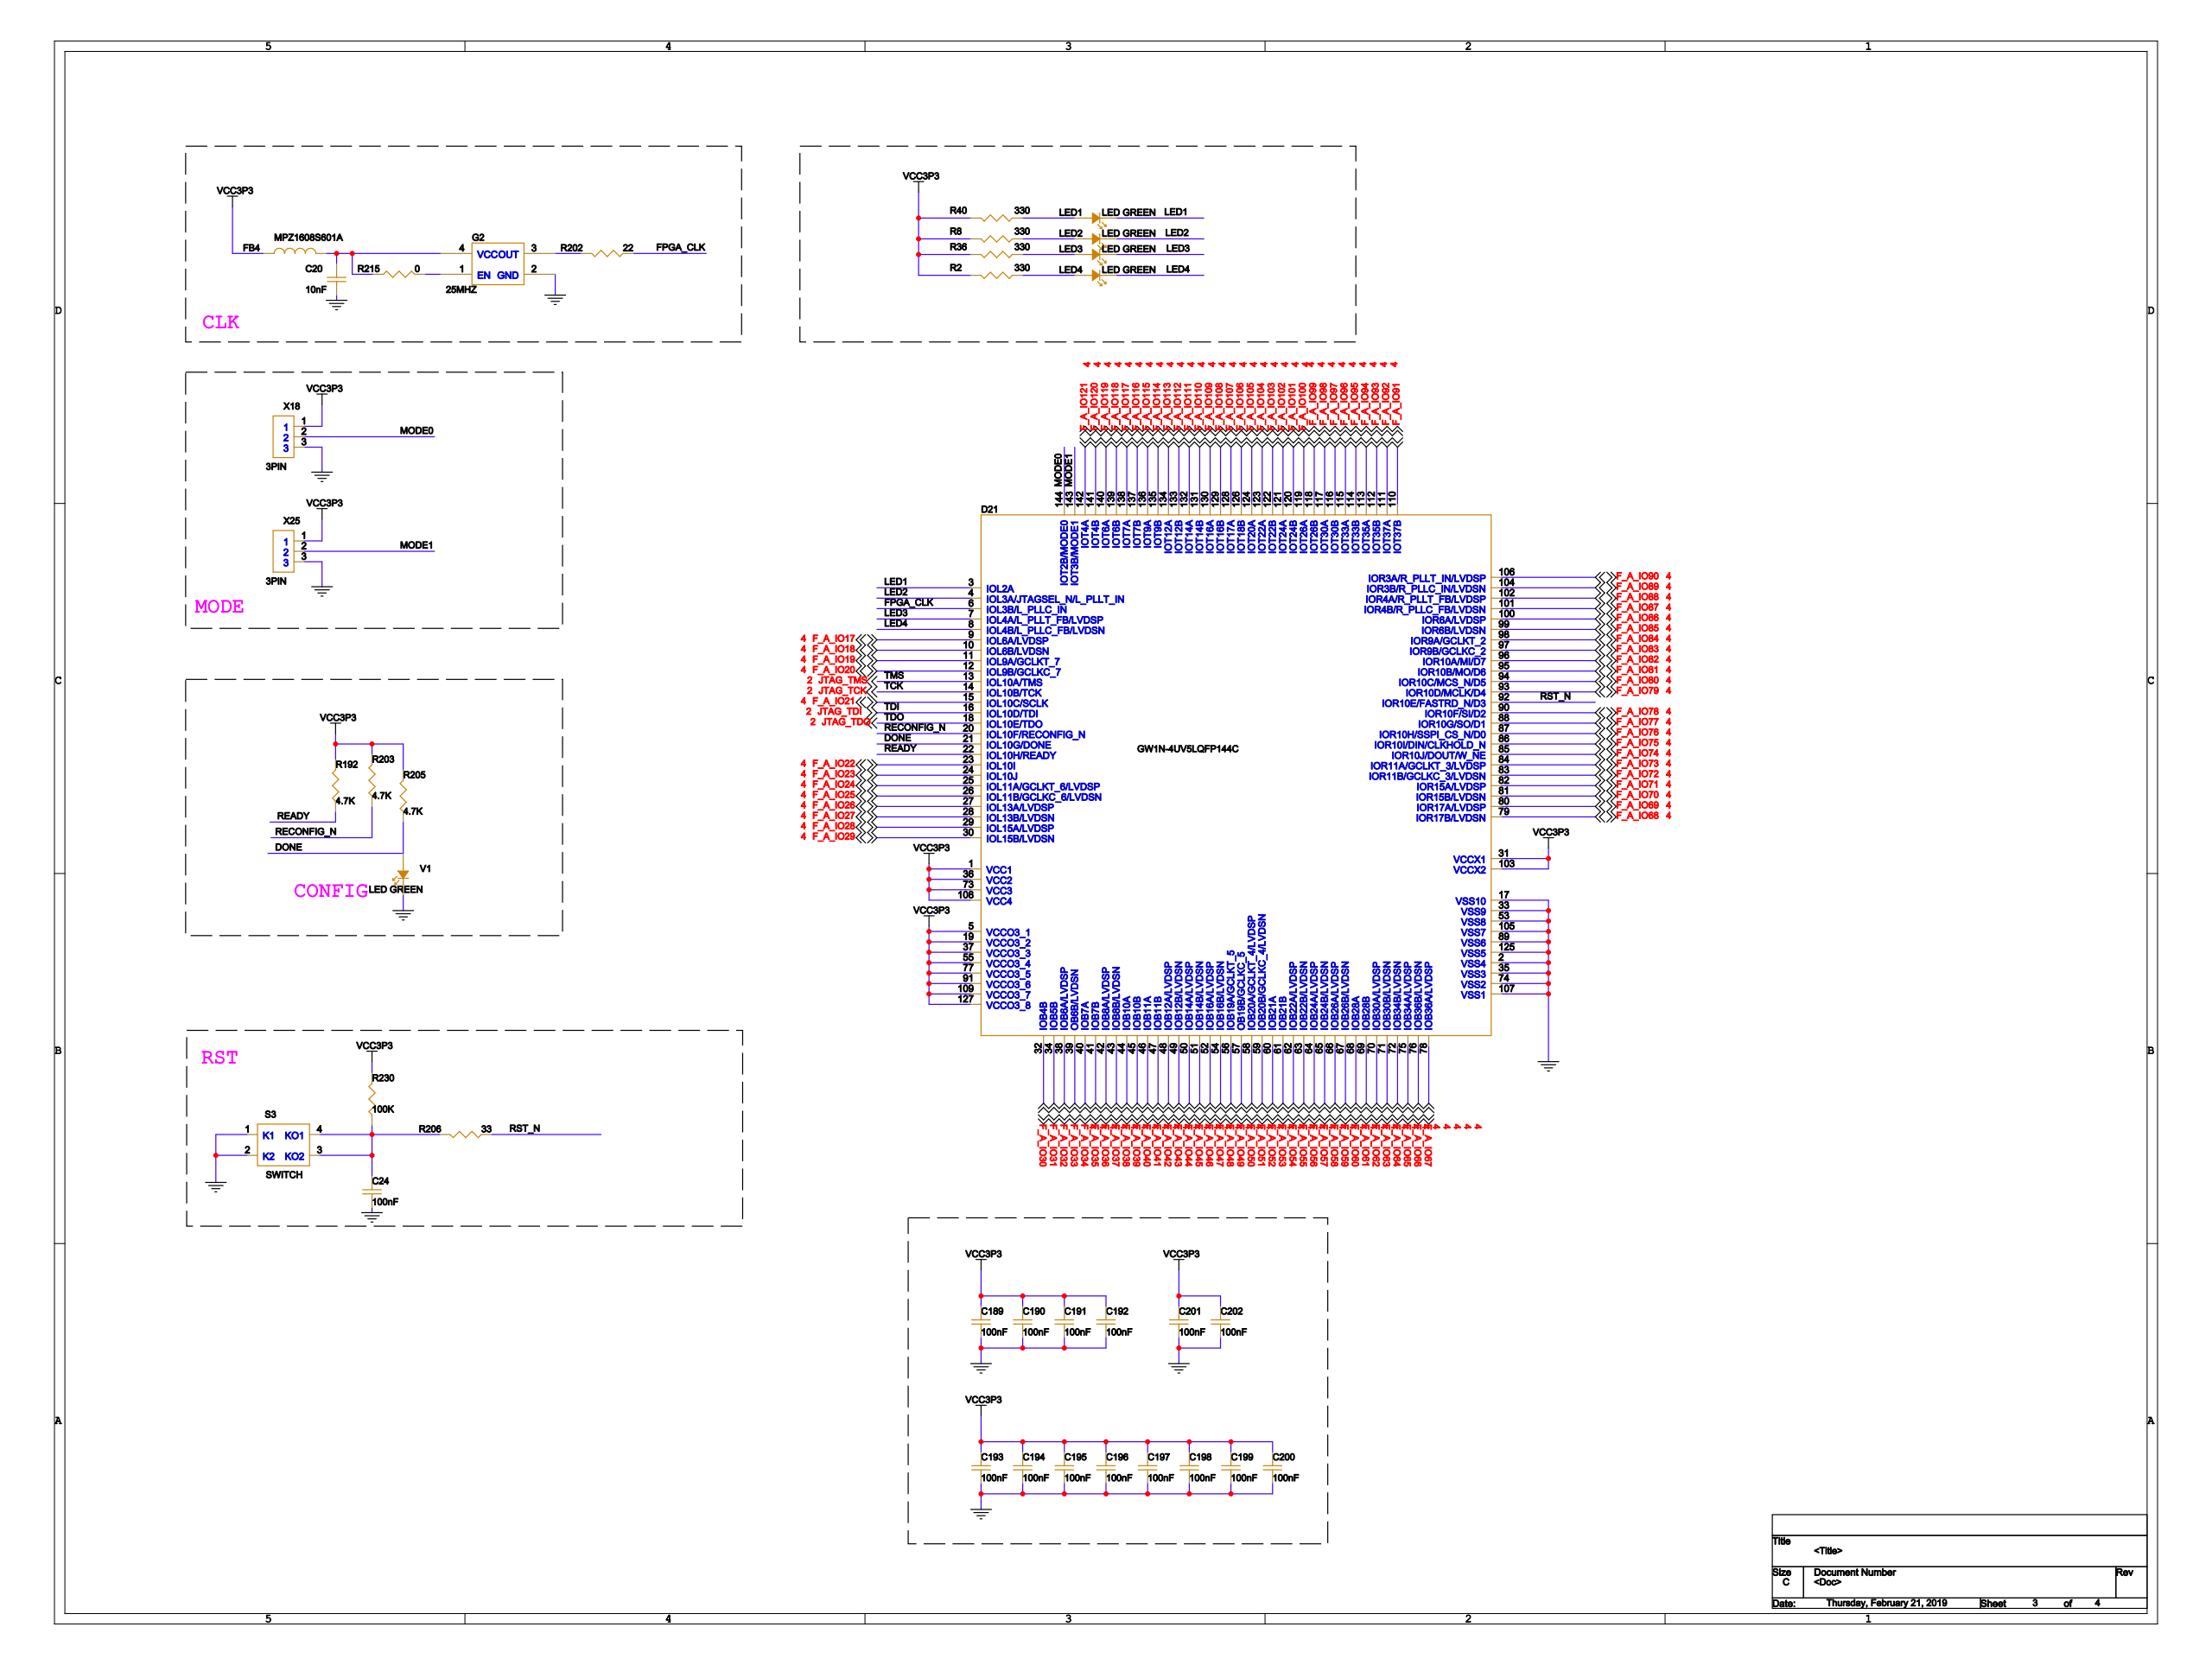Circuit board | Cadence Allegro | 174 parts | 250 nets | one sheet of the schematic
Parts on this sheet (reference | value | footprint):
C20 | 10nF | SMC0603
C24 | 100nF | SMC0603
C189 | 100nF | SMC0603
C190 | 100nF | SMC0603
C191 | 100nF | SMC0603
C192 | 100nF | SMC0603
C193 | 100nF | SMC0603
C194 | 100nF | SMC0603
C195 | 100nF | SMC0603
C196 | 100nF | SMC0603
C197 | 100nF | SMC0603
C198 | 100nF | SMC0603
C199 | 100nF | SMC0603
C200 | 100nF | SMC0603
C201 | 100nF | SMC0603
C202 | 100nF | SMC0603
D21 | GW1N-4UV5LQFP144C | QFP144-20X20-P0_5M
FB4 | MPZ1608S601A | FB0603
G2 | 25MHZ | OSC4-XO53
LED1 | LED GREEN | LED0603
LED2 | LED GREEN | LED0603
LED3 | LED GREEN | LED0603
LED4 | LED GREEN | LED0603
R2 | 330 | R0603
R8 | 330 | R0603
R36 | 330 | R0603
R40 | 330 | R0603
R192 | 4.7K | R0603
R202 | 22 | R0603
R203 | 4.7K | R0603
R205 | 4.7K | R0603
R206 | 33 | R0603
R215 | 0 | R0603
R230 | 100K | R0603
S3 | SWITCH | J-SW-4-9_1-E_SWITCH-TL330
V1 | LED GREEN | LED0603
X18 | 3PIN | SHDR1X3_254-HB11031
X25 | 3PIN | SHDR1X3_254-HB11031
Nets of these parts (net: part-pin ...):
GND: C20-2 C24-2 C189-2 C190-2 C191-2 C192-2 C193-2 C194-2 C195-2 C196-2 C197-2 C198-2 C199-2 C200-2 C201-2 C202-2 G2-2 S3-1 S3-2 V1-2 X18-3 X25-3 D21-2 D21-17 D21-33 D21-35 D21-53 D21-74 D21-89 D21-105 D21-107 D21-125
N2557374: C20-1 FB4-2 G2-4 R215-1
VCC3P3: C189-1 C190-1 C191-1 C192-1 C193-1 C194-1 C195-1 C196-1 C197-1 C198-1 C199-1 C200-1 C201-1 C202-1 FB4-1 R2-2 R8-2 R36-2 R40-2 R192-2 R203-2 R205-2 R230-2 X18-1 X25-1 D21-1 D21-5 D21-19 D21-31 D21-36 D21-37 D21-55 D21-73 D21-77 D21-91 D21-103 D21-108 D21-109 D21-127
N2559338: C24-1 R206-2 R230-1 S3-3 S3-4
F_A_IO30: D21-32
F_A_IO31: D21-34
F_A_IO32: D21-38
F_A_IO34: D21-40
JTAG_TMS: D21-13
JTAG_TCK: D21-14
F_A_IO21: D21-15
JTAG_TDI: D21-16
JTAG_TDO: D21-18
RECONFIG_N: R203-1 D21-20
DONE: R205-1 V1-1 D21-21
READY: R192-1 D21-22
F_A_IO22: D21-23
F_A_IO23: D21-24
F_A_IO24: D21-25
F_A_IO25: D21-26
F_A_IO26: D21-27
F_A_IO27: D21-28
F_A_IO28: D21-29
F_A_IO29: D21-30
LED1: LED1-2 D21-3
LED2: LED2-2 D21-4
FPGA_CLK: R202-1 D21-6
LED3: LED3-2 D21-7
LED4: LED4-2 D21-8
F_A_IO17: D21-9
F_A_IO18: D21-10
F_A_IO19: D21-11
F_A_IO20: D21-12
F_A_IO82: D21-96
F_A_IO81: D21-95
F_A_IO80: D21-94
F_A_IO79: D21-93
RST_N: R206-1 D21-92
F_A_IO78: D21-90
F_A_IO77: D21-88
F_A_IO76: D21-87
F_A_IO75: D21-86
F_A_IO74: D21-85
F_A_IO73: D21-84
F_A_IO72: D21-83
F_A_IO71: D21-82
F_A_IO70: D21-81
F_A_IO69: D21-80
F_A_IO68: D21-79
F_A_IO90: D21-106
F_A_IO89: D21-104
F_A_IO88: D21-102
F_A_IO87: D21-101
F_A_IO86: D21-100
F_A_IO85: D21-99
F_A_IO84: D21-98
F_A_IO83: D21-97
F_A_IO113: D21-134
F_A_IO112: D21-133
F_A_IO111: D21-132
F_A_IO110: D21-131
F_A_IO109: D21-130
F_A_IO108: D21-129
F_A_IO107: D21-128
F_A_IO106: D21-126
F_A_IO105: D21-124
F_A_IO104: D21-123
F_A_IO103: D21-122
F_A_IO102: D21-121
F_A_IO101: D21-120
F_A_IO100: D21-119
F_A_IO99: D21-118
MODE0: X18-2 D21-144
F_A_IO98: D21-117
F_A_IO97: D21-116
F_A_IO96: D21-115
F_A_IO95: D21-114
F_A_IO94: D21-113
F_A_IO93: D21-112
F_A_IO92: D21-111
F_A_IO91: D21-110
MODE1: X25-2 D21-143
F_A_IO121: D21-142
F_A_IO120: D21-141
F_A_IO119: D21-140
F_A_IO118: D21-139
F_A_IO117: D21-138
F_A_IO116: D21-137
F_A_IO115: D21-136
F_A_IO114: D21-135
F_A_IO33: D21-39
N2557462: G2-1 R215-2
N2557360: G2-3 R202-2
N2561355: LED1-1 R40-1
N2561381: LED2-1 R8-1
N2561439: LED3-1 R36-1
N2561481: LED4-1 R2-1